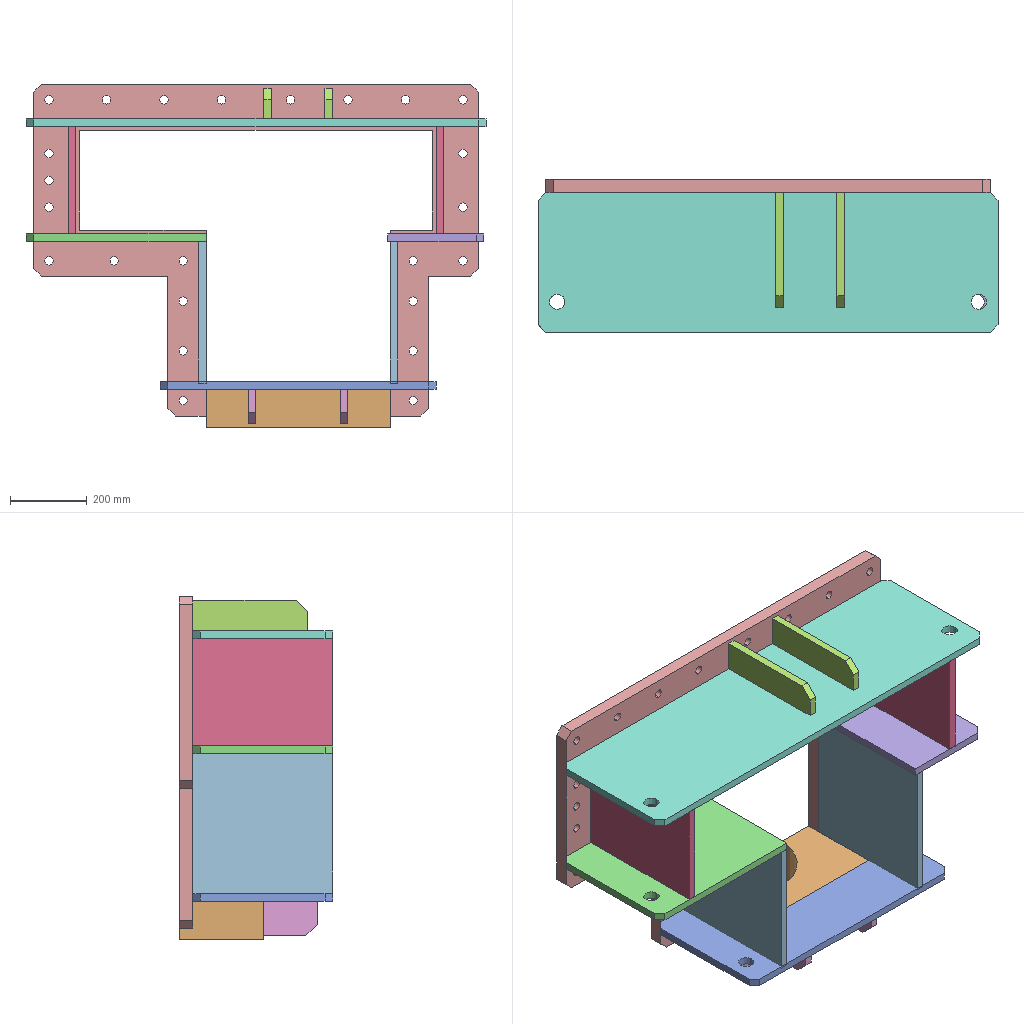Assembly | SolidWorks | 13 different items | 17 placed | box 1200 x 400 x 895 mm
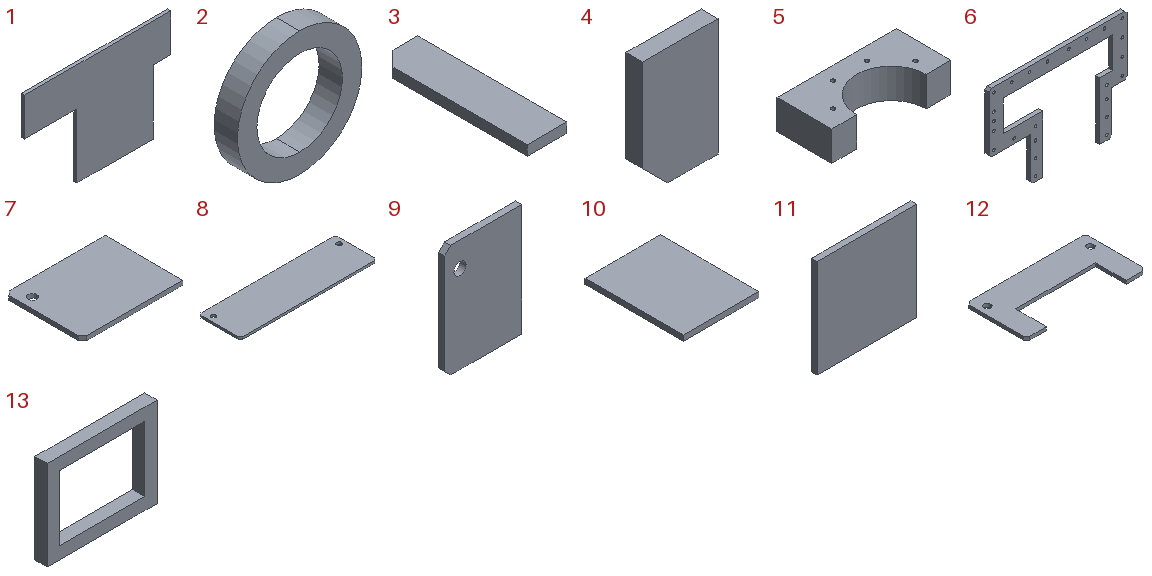Parts list (item | quantity | size | volume | features):
1 | x1 | 920 x 20 x 645 mm | 8304000 mm3 | features Extrusion 1
2 | x1 | 160 x 30 x 160 mm | 312871 mm3 | features Extrusion 1, HoleWzd 1
3 | x2 | 80 x 300 x 20 mm | 471000 mm3 | features Extrusion 1
4 | x2 | 90 x 20 x 140 mm | 243000 mm3 | features Extrusion 1
5 | x1 | 480 x 220 x 120 mm | 8956950 mm3 | features Extrusion 1, HoleWzd 1, RefAxis 1
6 | x1 | 1160 x 35 x 865 mm | 12105689 mm3 | features ICE 2, Chamfer 1, Extrusion 1
7 | x1 | 470 x 365 x 20 mm | 3397867 mm3 | features Chamfer 2, Extrusion 1, ICE 1
8 | x1 | 1200 x 365 x 20 mm | 8693735 mm3 | features Chamfer 2, Extrusion 1, ICE 1
9 | x1 | 250 x 20 x 365 mm | 1791867 mm3 | features Chamfer 2, Extrusion 1, ICE 1
10 | x2 | 280 x 365 x 20 mm | 2044000 mm3 | features Extrusion 1
11 | x2 | 369 x 20 x 365 mm | 2693700 mm3 | features Extrusion 1
12 | x1 | 720 x 365 x 20 mm | 3413735 mm3 | features Chamfer 2, ICE 2, Extrusion 1
13 | x1 | 270 x 30 x 220 mm | 767460 mm3 | features Extrusion 1, HoleWzd 1
Mates (type | each side: item.copy, entity, surface, feature):
Coincident | 6.1 face plane Boss-Extrude1 | 12.1 face plane Boss-Extrude1
Width | 12.1 face plane Boss-Extrude1 | 12.1 face plane Boss-Extrude1 | 6.1 face plane Boss-Extrude1 | 6.1 face plane Boss-Extrude1
Width | 5.1 face plane Boss-Extrude1 | 5.1 face plane Boss-Extrude1 | 6.1 face plane Boss-Extrude1 | 6.1 face plane Boss-Extrude1
Coincident | 6.1 face plane Boss-Extrude1 | 5.1 face plane Boss-Extrude1
Coincident | 4.1 face plane Boss-Extrude1 | 5.1 face plane Boss-Extrude1
Coincident | 12.1 face plane Boss-Extrude1 | 4.1 face plane Boss-Extrude1
DistanceDim | 5.1 axis | 4.1 face plane Boss-Extrude1
Coincident | 6.1 face plane Boss-Extrude1 | 3.1 face plane Boss-Extrude1
DistanceDim | 5.1 axis | 3.1 face plane Boss-Extrude1
Coincident | 6.1 face plane Boss-Extrude1 | 9.1 face plane Boss-Extrude1
Coincident | 6.1 face plane Boss-Extrude1 | 7.1 face plane Boss-Extrude1
Coincident | 6.1 face plane Boss-Extrude1 | 10.1 face plane Boss-Extrude1
DistanceDim | 5.1 face plane Boss-Extrude1 | 6.1 face plane Boss-Extrude1
Coincident | 3.1 face plane Boss-Extrude1 | 8.1 face plane Boss-Extrude1 | 2 times
DistanceDim | 8.1 face plane Boss-Extrude1 | 6.1 face plane Cut-Extrude1
Width | 8.1 face plane Boss-Extrude1 | 8.1 face plane Boss-Extrude1 | 6.1 face plane Boss-Extrude1 | 6.1 face plane Boss-Extrude1
Coincident | 6.1 face plane Boss-Extrude1 | 11.1 face plane Boss-Extrude1 | 2 times
Coincident | 9.1 face plane Boss-Extrude1 | 11.1 face plane Boss-Extrude1
Coincident | 6.1 face plane Boss-Extrude1 | 11.2 face plane Boss-Extrude1 | 2 times
Coincident | 7.1 face plane Boss-Extrude1 | 11.2 face plane Boss-Extrude1 | 2 times
Coincident | 8.1 face plane Boss-Extrude1 | 10.1 face plane Boss-Extrude1
Coincident | 7.1 face plane Boss-Extrude1 | 10.1 face plane Boss-Extrude1
Coincident | 6.1 face plane Boss-Extrude1 | 10.2 face plane Boss-Extrude1
Coincident | 9.1 face plane Boss-Extrude1 | 10.2 face plane Boss-Extrude1
Coincident | 8.1 face plane Boss-Extrude1 | 10.2 face plane Boss-Extrude1
DistanceDim | 10.1 face plane Boss-Extrude1 | 6.1 face plane Cut-Extrude1
DistanceDim | 6.1 face plane Cut-Extrude1 | 10.2 face plane Boss-Extrude1
Coincident | 12.1 face plane Boss-Extrude1 | 5.1 face plane Boss-Extrude1